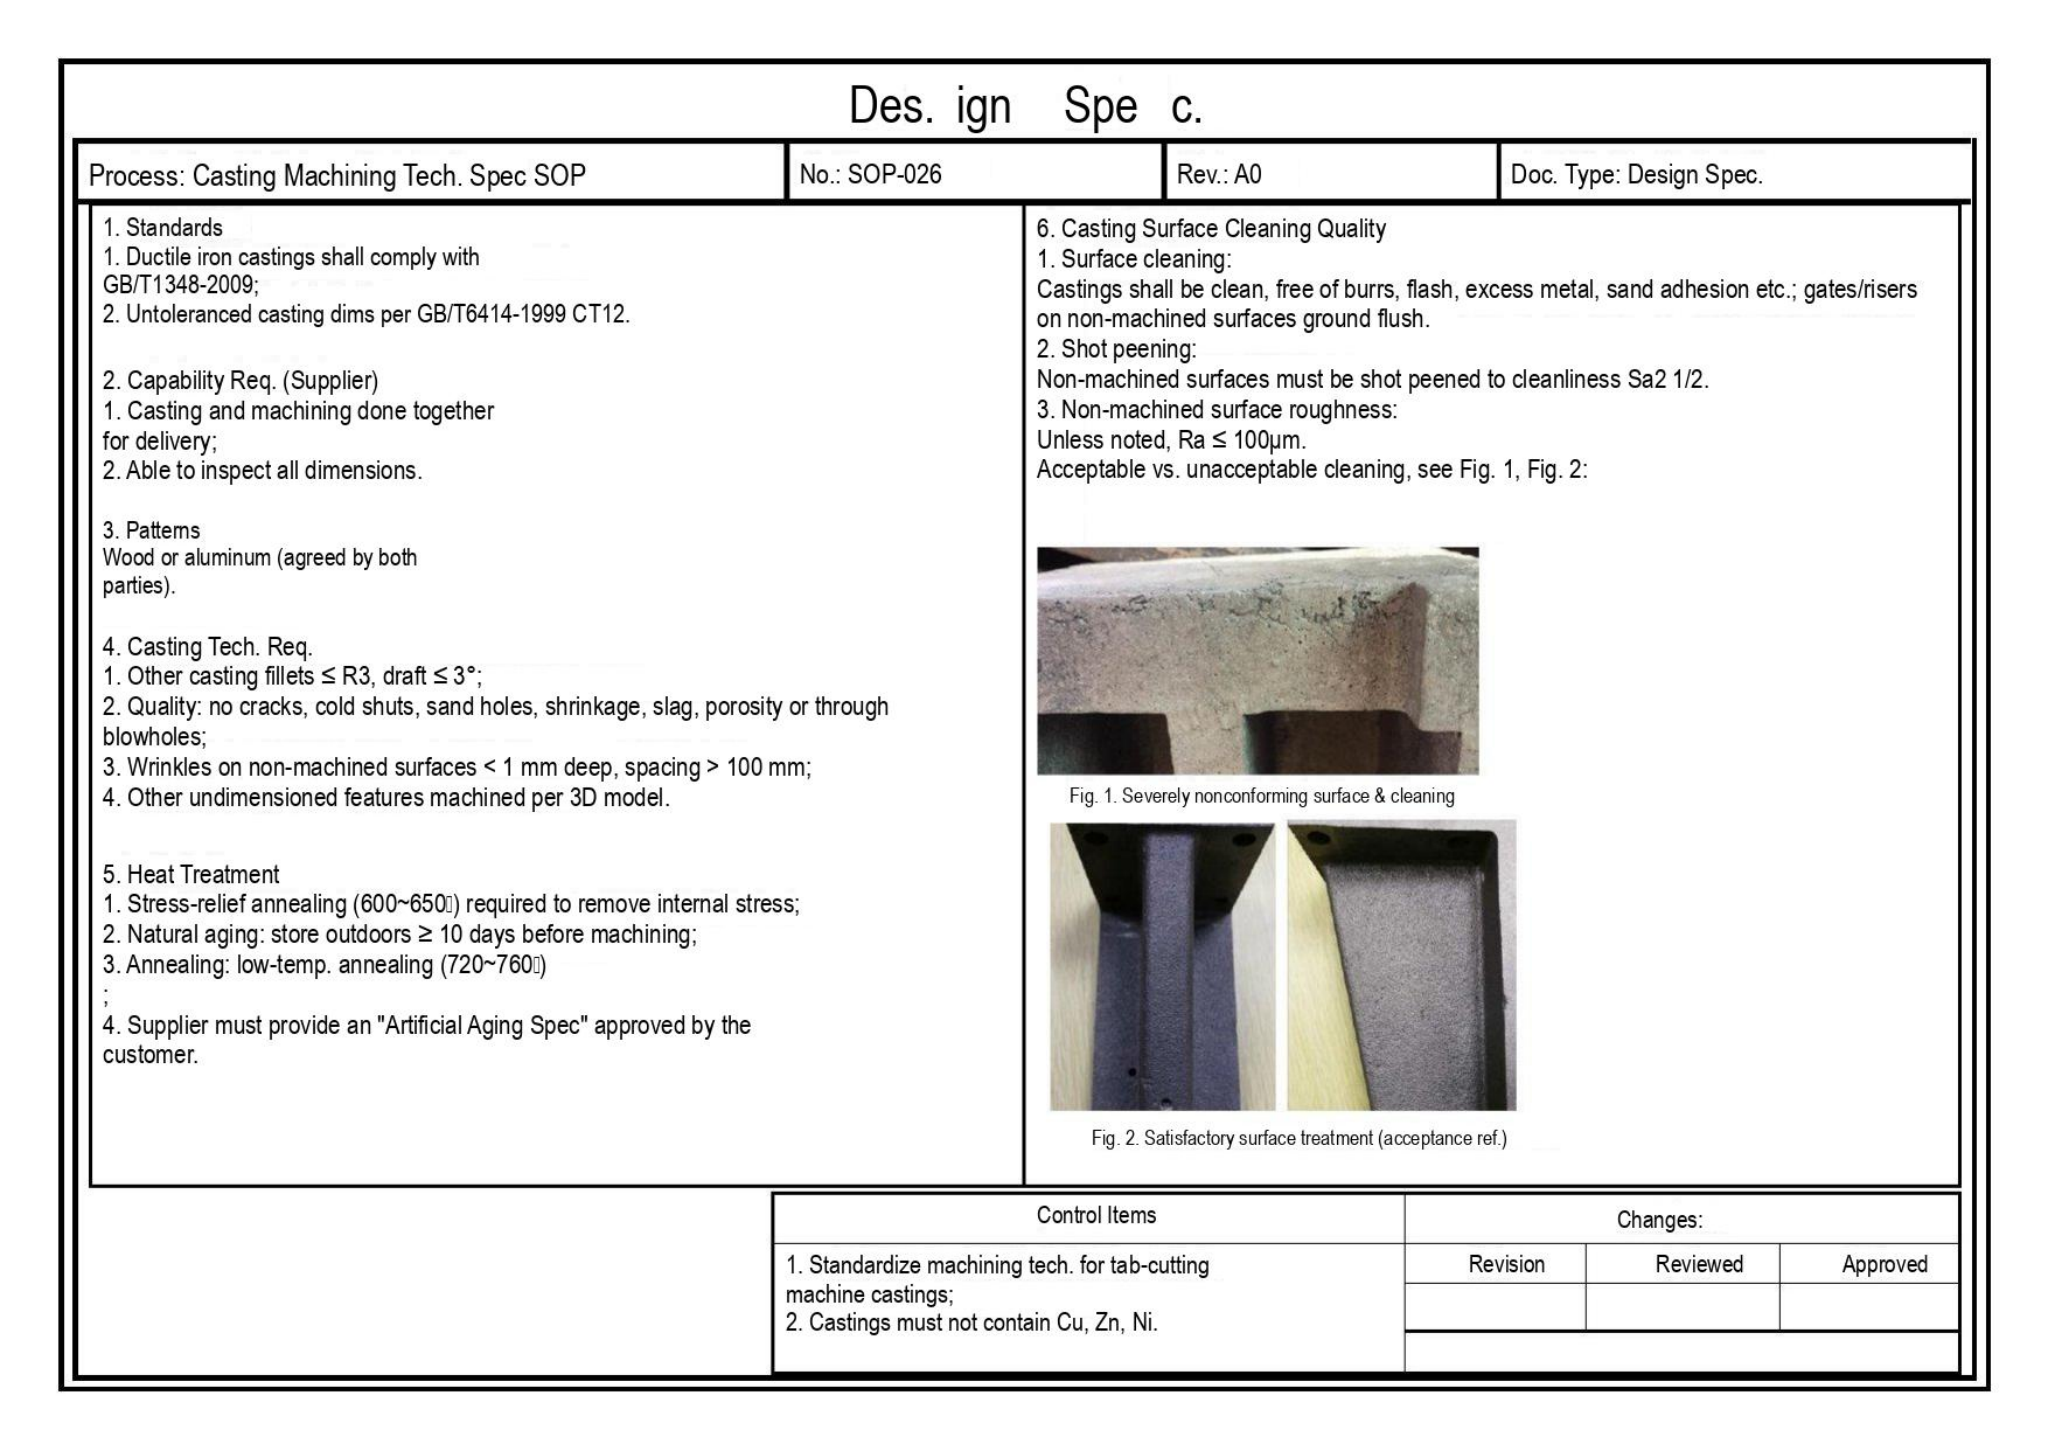Des. ign Spe c.

| Process: Casting Machining Tech. Spec SOP | No.: SOP-026 | Rev.: A0 | Doc. Type: Design Spec. |
|---|---|---|---|

1. Standards
1. Ductile iron castings shall comply with GB/T1348-2009;
2. Untoleranced casting dims per GB/T6414-1999 CT12.

2. Capability Req. (Supplier)
1. Casting and machining done together for delivery;
2. Able to inspect all dimensions.

3. Patterns
Wood or aluminum (agreed by both parties).

4. Casting Tech. Req.
1. Other casting fillets ≤ R3, draft ≤ 3°;
2. Quality: no cracks, cold shuts, sand holes, shrinkage, slag, porosity or through blowholes;
3. Wrinkles on non-machined surfaces < 1 mm deep, spacing > 100 mm;
4. Other undimensioned features machined per 3D model.

5. Heat Treatment
1. Stress-relief annealing (600~650) required to remove internal stress;
2. Natural aging: store outdoors ≥ 10 days before machining;
3. Annealing: low-temp. annealing (720~760)
;
4. Supplier must provide an "Artificial Aging Spec" approved by the customer.

6. Casting Surface Cleaning Quality
1. Surface cleaning:
Castings shall be clean, free of burrs, flash, excess metal, sand adhesion etc.; gates/risers on non-machined surfaces ground flush.
2. Shot peening:
Non-machined surfaces must be shot peened to cleanliness Sa2 1/2.
3. Non-machined surface roughness:
Unless noted, Ra ≤ 100μm.
Acceptable vs. unacceptable cleaning, see Fig. 1, Fig. 2:

Fig. 1. Severely nonconforming surface & cleaning

Fig. 2. Satisfactory surface treatment (acceptance ref.)

| Control Items | Changes: | | |
|---|---|---|---|
| 1. Standardize machining tech. for tab-cutting machine castings;<br>2. Castings must not contain Cu, Zn, Ni. | Revision | Reviewed | Approved |
| | | | |
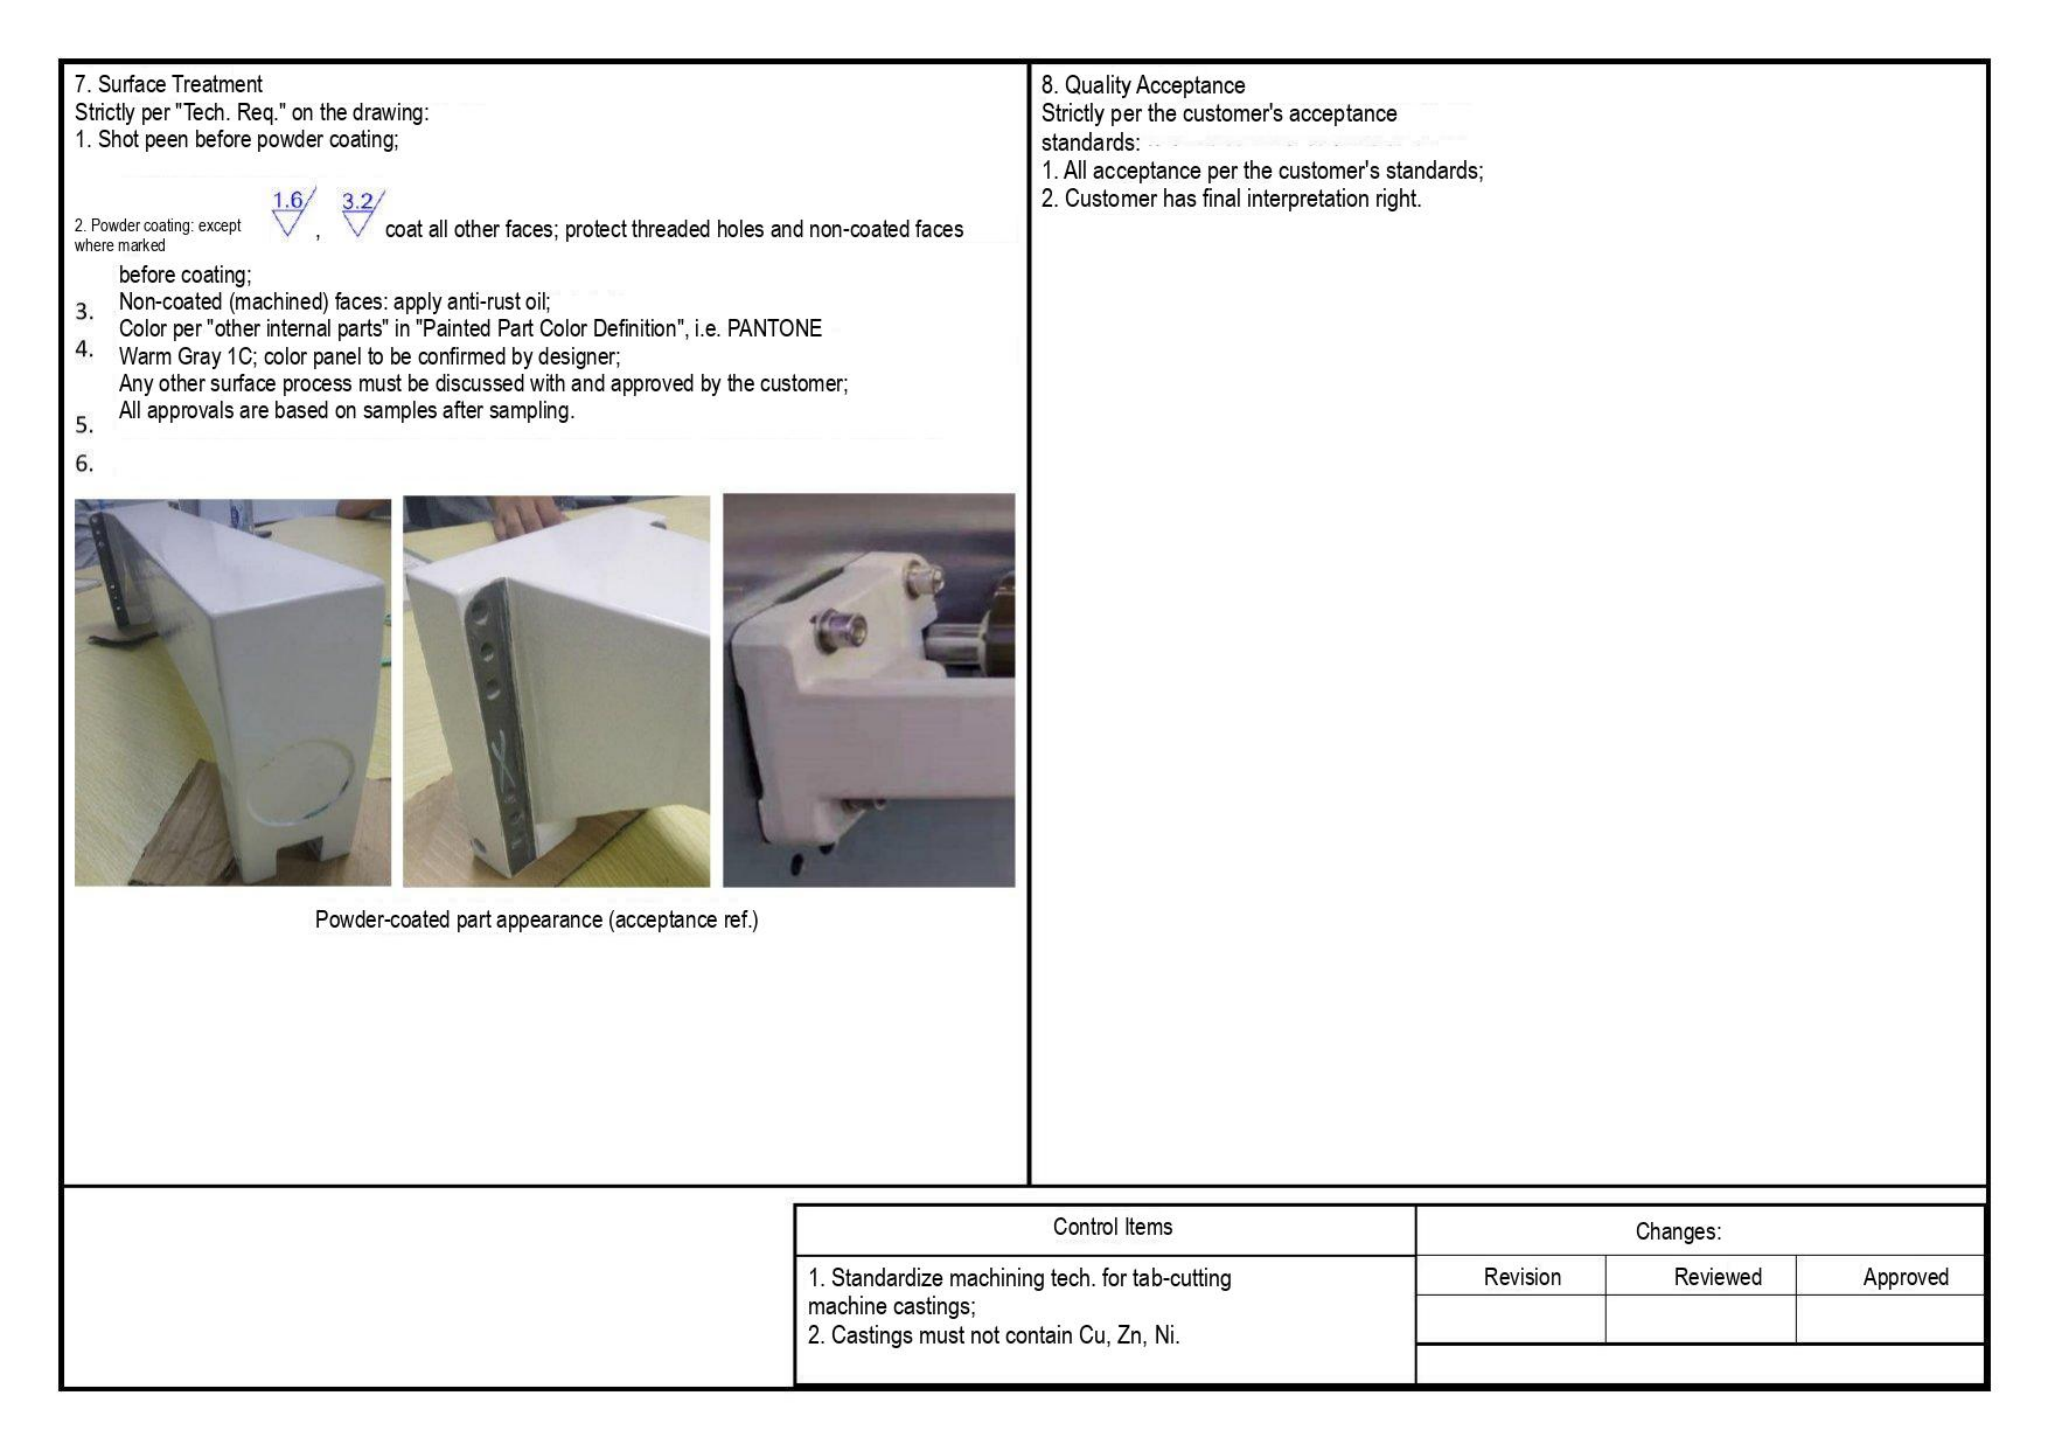7. Surface Treatment
Strictly per "Tech. Req." on the drawing:
1. Shot peen before powder coating;
2. Powder coating: except where marked 1.6, 3.2 coat all other faces; protect threaded holes and non-coated faces before coating;
3. Non-coated (machined) faces: apply anti-rust oil;
4. Color per "other internal parts" in "Painted Part Color Definition", i.e. PANTONE Warm Gray 1C; color panel to be confirmed by designer;
5. Any other surface process must be discussed with and approved by the customer;
6. All approvals are based on samples after sampling.

Powder-coated part appearance (acceptance ref.)

8. Quality Acceptance
Strictly per the customer's acceptance standards:
1. All acceptance per the customer's standards;
2. Customer has final interpretation right.

| Control Items | Changes: | | |
|---|---|---|---|
| 1. Standardize machining tech. for tab-cutting machine castings;<br>2. Castings must not contain Cu, Zn, Ni. | Revision | Reviewed | Approved |
| | | | |